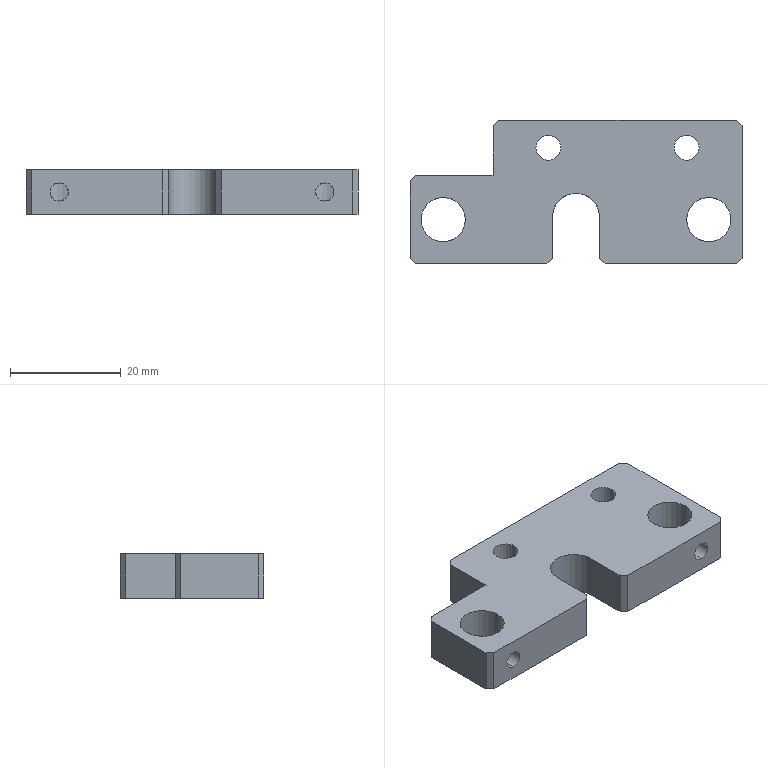Part | SolidWorks | features ICE 3, HoleWzd 2, Chamfer 1, Extrusion 1 | 1 solid | 31 faces | box 60 x 26 x 8 mm | volume 9318 mm3 | plane 18 | cylinder 13 | commonest cylinder face diameters 3.3 x4 4.5 x4 8 x4 8.5 x1
STEP:
#1=CARTESIAN_POINT('',(-2.75,21.,8.));
#2=VERTEX_POINT('',#1);
#3=CARTESIAN_POINT('',(-7.25,21.,8.));
#4=VERTEX_POINT('',#3);
#5=CARTESIAN_POINT('',(-5.,21.,8.));
#6=DIRECTION('',(0.,0.,-1.));
#7=DIRECTION('',(-1.,0.,0.));
#8=AXIS2_PLACEMENT_3D('',#5,#6,#7);
#9=CIRCLE('',#8,2.25);
#10=EDGE_CURVE('',#2,#4,#9,.T.);
#11=ORIENTED_EDGE('',*,*,#10,.F.);
#12=CARTESIAN_POINT('',(-2.75,21.,0.));
#13=VERTEX_POINT('',#12);
#14=CARTESIAN_POINT('',(-2.75,21.,8.));
#15=DIRECTION('',(0.,0.,-1.));
#16=VECTOR('',#15,1000.);
#17=LINE('',#14,#16);
#18=EDGE_CURVE('',#2,#13,#17,.T.);
#19=ORIENTED_EDGE('',*,*,#18,.T.);
#20=CARTESIAN_POINT('',(-7.25,21.,0.));
#21=VERTEX_POINT('',#20);
#22=CARTESIAN_POINT('',(-5.,21.,0.));
#23=DIRECTION('',(0.,0.,-1.));
#24=DIRECTION('',(-1.,0.,0.));
#25=AXIS2_PLACEMENT_3D('',#22,#23,#24);
#26=CIRCLE('',#25,2.25);
#27=EDGE_CURVE('',#13,#21,#26,.T.);
#28=ORIENTED_EDGE('',*,*,#27,.T.);
#29=CARTESIAN_POINT('',(-7.25,21.,8.));
#30=DIRECTION('',(0.,0.,-1.));
#31=VECTOR('',#30,1000.);
#32=LINE('',#29,#31);
#33=EDGE_CURVE('',#4,#21,#32,.T.);
#34=ORIENTED_EDGE('',*,*,#33,.F.);
#35=EDGE_LOOP('',(#11,#19,#28,#34));
#36=FACE_OUTER_BOUND('',#35,.T.);
#37=CARTESIAN_POINT('',(-5.,21.,8.));
#38=DIRECTION('',(0.,0.,-1.));
#39=DIRECTION('',(-1.,0.,0.));
#40=AXIS2_PLACEMENT_3D('',#37,#38,#39);
#41=CYLINDRICAL_SURFACE('',#40,2.25);
#42=ADVANCED_FACE('',(#36),#41,.F.);
#43=CARTESIAN_POINT('',(22.25,21.,8.));
#44=VERTEX_POINT('',#43);
#45=CARTESIAN_POINT('',(17.75,21.,8.));
#46=VERTEX_POINT('',#45);
#47=CARTESIAN_POINT('',(20.,21.,8.));
#48=DIRECTION('',(0.,0.,-1.));
#49=DIRECTION('',(-1.,0.,0.));
#50=AXIS2_PLACEMENT_3D('',#47,#48,#49);
#51=CIRCLE('',#50,2.25);
#52=EDGE_CURVE('',#44,#46,#51,.T.);
#53=ORIENTED_EDGE('',*,*,#52,.F.);
#54=CARTESIAN_POINT('',(22.25,21.,0.));
#55=VERTEX_POINT('',#54);
#56=CARTESIAN_POINT('',(22.25,21.,8.));
#57=DIRECTION('',(0.,0.,-1.));
#58=VECTOR('',#57,1000.);
#59=LINE('',#56,#58);
#60=EDGE_CURVE('',#44,#55,#59,.T.);
#61=ORIENTED_EDGE('',*,*,#60,.T.);
#62=CARTESIAN_POINT('',(17.75,21.,0.));
#63=VERTEX_POINT('',#62);
#64=CARTESIAN_POINT('',(20.,21.,0.));
#65=DIRECTION('',(0.,0.,-1.));
#66=DIRECTION('',(-1.,0.,0.));
#67=AXIS2_PLACEMENT_3D('',#64,#65,#66);
#68=CIRCLE('',#67,2.25);
#69=EDGE_CURVE('',#55,#63,#68,.T.);
#70=ORIENTED_EDGE('',*,*,#69,.T.);
#71=CARTESIAN_POINT('',(17.75,21.,8.));
#72=DIRECTION('',(0.,0.,-1.));
#73=VECTOR('',#72,1000.);
#74=LINE('',#71,#73);
#75=EDGE_CURVE('',#46,#63,#74,.T.);
#76=ORIENTED_EDGE('',*,*,#75,.F.);
#77=EDGE_LOOP('',(#53,#61,#70,#76));
#78=FACE_OUTER_BOUND('',#77,.T.);
#79=CARTESIAN_POINT('',(20.,21.,8.));
#80=DIRECTION('',(0.,0.,-1.));
#81=DIRECTION('',(-1.,0.,0.));
#82=AXIS2_PLACEMENT_3D('',#79,#80,#81);
#83=CYLINDRICAL_SURFACE('',#82,2.25);
#84=ADVANCED_FACE('',(#78),#83,.F.);
#85=CARTESIAN_POINT('',(-24.,4.,2.35));
#86=VERTEX_POINT('',#85);
#87=CARTESIAN_POINT('',(-24.,4.,5.65));
#88=VERTEX_POINT('',#87);
#89=CARTESIAN_POINT('',(-24.,4.,2.35));
#90=CARTESIAN_POINT('',(-24.11,4.,2.35));
#91=CARTESIAN_POINT('',(-24.219,4.005,2.361));
#92=CARTESIAN_POINT('',(-24.431,4.022,2.404));
#93=CARTESIAN_POINT('',(-24.537,4.035,2.436));
#94=CARTESIAN_POINT('',(-24.836,4.083,2.561));
#95=CARTESIAN_POINT('',(-25.017,4.128,2.684));
#96=CARTESIAN_POINT('',(-25.318,4.22,2.985));
#97=CARTESIAN_POINT('',(-25.44,4.267,3.166));
#98=CARTESIAN_POINT('',(-25.564,4.318,3.463));
#99=CARTESIAN_POINT('',(-25.596,4.332,3.568));
#100=CARTESIAN_POINT('',(-25.639,4.351,3.782));
#101=CARTESIAN_POINT('',(-25.65,4.356,3.89));
#102=CARTESIAN_POINT('',(-25.65,4.356,4.108));
#103=CARTESIAN_POINT('',(-25.639,4.351,4.219));
#104=CARTESIAN_POINT('',(-25.596,4.332,4.431));
#105=CARTESIAN_POINT('',(-25.565,4.318,4.535));
#106=CARTESIAN_POINT('',(-25.481,4.284,4.736));
#107=CARTESIAN_POINT('',(-25.43,4.264,4.83));
#108=CARTESIAN_POINT('',(-25.311,4.22,5.008));
#109=CARTESIAN_POINT('',(-25.242,4.197,5.092));
#110=CARTESIAN_POINT('',(-25.091,4.151,5.243));
#111=CARTESIAN_POINT('',(-25.009,4.128,5.31));
#112=CARTESIAN_POINT('',(-24.83,4.086,5.43));
#113=CARTESIAN_POINT('',(-24.734,4.067,5.481));
#114=CARTESIAN_POINT('',(-24.437,4.019,5.606));
#115=CARTESIAN_POINT('',(-24.217,4.,5.65));
#116=CARTESIAN_POINT('',(-24.,4.,5.65));
#117=B_SPLINE_CURVE_WITH_KNOTS('',3,(#89,#90,#91,#92,#93,#94,#95,#96,#97,#98,#99,#100,#101,#102,#103,#104,#105,#106,#107,#108,#109,#110,#111,#112,#113,#114,#115,#116),.UNSPECIFIED.,.F.,.F.,(4,2,2,2,2,2,2,2,2,2,2,2,2,4),(0.,0.0003261,0.0006522,0.001304,0.001957,0.002283,0.002609,0.002935,0.003261,0.003587,0.003913,0.004239,0.004565,0.005218),.UNSPECIFIED.);
#118=EDGE_CURVE('',#86,#88,#117,.T.);
#119=ORIENTED_EDGE('',*,*,#118,.T.);
#120=CARTESIAN_POINT('',(-24.,0.,5.65));
#121=VERTEX_POINT('',#120);
#122=CARTESIAN_POINT('',(-24.,0.,5.65));
#123=DIRECTION('',(0.,-1.,0.));
#124=VECTOR('',#123,1000.);
#125=LINE('',#122,#124);
#126=EDGE_CURVE('',#88,#121,#125,.T.);
#127=ORIENTED_EDGE('',*,*,#126,.T.);
#128=CARTESIAN_POINT('',(-24.,0.,2.35));
#129=VERTEX_POINT('',#128);
#130=CARTESIAN_POINT('',(-24.,0.,4.));
#131=DIRECTION('',(0.,-1.,0.));
#132=DIRECTION('',(0.,0.,-1.));
#133=AXIS2_PLACEMENT_3D('',#130,#131,#132);
#134=CIRCLE('',#133,1.65);
#135=EDGE_CURVE('',#121,#129,#134,.T.);
#136=ORIENTED_EDGE('',*,*,#135,.T.);
#137=CARTESIAN_POINT('',(-24.,0.,2.35));
#138=DIRECTION('',(0.,-1.,0.));
#139=VECTOR('',#138,1000.);
#140=LINE('',#137,#139);
#141=EDGE_CURVE('',#86,#129,#140,.T.);
#142=ORIENTED_EDGE('',*,*,#141,.F.);
#143=EDGE_LOOP('',(#119,#127,#136,#142));
#144=FACE_OUTER_BOUND('',#143,.T.);
#145=CARTESIAN_POINT('',(-24.,0.,4.));
#146=DIRECTION('',(0.,-1.,0.));
#147=DIRECTION('',(0.,0.,-1.));
#148=AXIS2_PLACEMENT_3D('',#145,#146,#147);
#149=CYLINDRICAL_SURFACE('',#148,1.65);
#150=ADVANCED_FACE('',(#144),#149,.F.);
#151=CARTESIAN_POINT('',(24.,4.,2.35));
#152=VERTEX_POINT('',#151);
#153=CARTESIAN_POINT('',(24.,4.,5.65));
#154=VERTEX_POINT('',#153);
#155=CARTESIAN_POINT('',(24.,4.,2.35));
#156=CARTESIAN_POINT('',(23.89,4.,2.35));
#157=CARTESIAN_POINT('',(23.781,4.005,2.361));
#158=CARTESIAN_POINT('',(23.569,4.022,2.404));
#159=CARTESIAN_POINT('',(23.463,4.035,2.436));
#160=CARTESIAN_POINT('',(23.164,4.083,2.561));
#161=CARTESIAN_POINT('',(22.983,4.128,2.684));
#162=CARTESIAN_POINT('',(22.682,4.22,2.985));
#163=CARTESIAN_POINT('',(22.56,4.267,3.166));
#164=CARTESIAN_POINT('',(22.436,4.318,3.463));
#165=CARTESIAN_POINT('',(22.404,4.332,3.568));
#166=CARTESIAN_POINT('',(22.361,4.351,3.782));
#167=CARTESIAN_POINT('',(22.35,4.356,3.89));
#168=CARTESIAN_POINT('',(22.35,4.356,4.108));
#169=CARTESIAN_POINT('',(22.361,4.351,4.219));
#170=CARTESIAN_POINT('',(22.404,4.332,4.431));
#171=CARTESIAN_POINT('',(22.435,4.318,4.535));
#172=CARTESIAN_POINT('',(22.519,4.284,4.736));
#173=CARTESIAN_POINT('',(22.57,4.264,4.83));
#174=CARTESIAN_POINT('',(22.689,4.22,5.008));
#175=CARTESIAN_POINT('',(22.758,4.197,5.092));
#176=CARTESIAN_POINT('',(22.909,4.151,5.243));
#177=CARTESIAN_POINT('',(22.991,4.128,5.31));
#178=CARTESIAN_POINT('',(23.17,4.086,5.43));
#179=CARTESIAN_POINT('',(23.266,4.067,5.481));
#180=CARTESIAN_POINT('',(23.563,4.019,5.606));
#181=CARTESIAN_POINT('',(23.783,4.,5.65));
#182=CARTESIAN_POINT('',(24.,4.,5.65));
#183=B_SPLINE_CURVE_WITH_KNOTS('',3,(#155,#156,#157,#158,#159,#160,#161,#162,#163,#164,#165,#166,#167,#168,#169,#170,#171,#172,#173,#174,#175,#176,#177,#178,#179,#180,#181,#182),.UNSPECIFIED.,.F.,.F.,(4,2,2,2,2,2,2,2,2,2,2,2,2,4),(0.,0.0003261,0.0006522,0.001304,0.001957,0.002283,0.002609,0.002935,0.003261,0.003587,0.003913,0.004239,0.004565,0.005218),.UNSPECIFIED.);
#184=EDGE_CURVE('',#152,#154,#183,.T.);
#185=ORIENTED_EDGE('',*,*,#184,.T.);
#186=CARTESIAN_POINT('',(24.,0.,5.65));
#187=VERTEX_POINT('',#186);
#188=CARTESIAN_POINT('',(24.,0.,5.65));
#189=DIRECTION('',(0.,-1.,0.));
#190=VECTOR('',#189,1000.);
#191=LINE('',#188,#190);
#192=EDGE_CURVE('',#154,#187,#191,.T.);
#193=ORIENTED_EDGE('',*,*,#192,.T.);
#194=CARTESIAN_POINT('',(24.,0.,2.35));
#195=VERTEX_POINT('',#194);
#196=CARTESIAN_POINT('',(24.,0.,4.));
#197=DIRECTION('',(0.,-1.,0.));
#198=DIRECTION('',(0.,0.,-1.));
#199=AXIS2_PLACEMENT_3D('',#196,#197,#198);
#200=CIRCLE('',#199,1.65);
#201=EDGE_CURVE('',#187,#195,#200,.T.);
#202=ORIENTED_EDGE('',*,*,#201,.T.);
#203=CARTESIAN_POINT('',(24.,0.,2.35));
#204=DIRECTION('',(0.,-1.,0.));
#205=VECTOR('',#204,1000.);
#206=LINE('',#203,#205);
#207=EDGE_CURVE('',#152,#195,#206,.T.);
#208=ORIENTED_EDGE('',*,*,#207,.F.);
#209=EDGE_LOOP('',(#185,#193,#202,#208));
#210=FACE_OUTER_BOUND('',#209,.T.);
#211=CARTESIAN_POINT('',(24.,0.,4.));
#212=DIRECTION('',(0.,-1.,0.));
#213=DIRECTION('',(0.,0.,-1.));
#214=AXIS2_PLACEMENT_3D('',#211,#212,#213);
#215=CYLINDRICAL_SURFACE('',#214,1.65);
#216=ADVANCED_FACE('',(#210),#215,.F.);
#217=ORIENTED_EDGE('',*,*,#184,.F.);
#218=CARTESIAN_POINT('',(24.,4.,5.65));
#219=CARTESIAN_POINT('',(24.109,4.,5.65));
#220=CARTESIAN_POINT('',(24.219,4.005,5.639));
#221=CARTESIAN_POINT('',(24.433,4.022,5.596));
#222=CARTESIAN_POINT('',(24.536,4.035,5.564));
#223=CARTESIAN_POINT('',(24.835,4.083,5.439));
#224=CARTESIAN_POINT('',(25.016,4.128,5.318));
#225=CARTESIAN_POINT('',(25.244,4.197,5.09));
#226=CARTESIAN_POINT('',(25.311,4.22,5.008));
#227=CARTESIAN_POINT('',(25.43,4.264,4.83));
#228=CARTESIAN_POINT('',(25.481,4.284,4.734));
#229=CARTESIAN_POINT('',(25.564,4.318,4.535));
#230=CARTESIAN_POINT('',(25.596,4.332,4.433));
#231=CARTESIAN_POINT('',(25.639,4.351,4.22));
#232=CARTESIAN_POINT('',(25.65,4.356,4.109));
#233=CARTESIAN_POINT('',(25.65,4.356,3.783));
#234=CARTESIAN_POINT('',(25.606,4.335,3.564));
#235=CARTESIAN_POINT('',(25.482,4.284,3.266));
#236=CARTESIAN_POINT('',(25.43,4.264,3.17));
#237=CARTESIAN_POINT('',(25.311,4.22,2.992));
#238=CARTESIAN_POINT('',(25.243,4.197,2.91));
#239=CARTESIAN_POINT('',(25.092,4.151,2.758));
#240=CARTESIAN_POINT('',(25.008,4.128,2.689));
#241=CARTESIAN_POINT('',(24.831,4.086,2.571));
#242=CARTESIAN_POINT('',(24.737,4.067,2.52));
#243=CARTESIAN_POINT('',(24.435,4.018,2.393));
#244=CARTESIAN_POINT('',(24.221,4.,2.35));
#245=CARTESIAN_POINT('',(24.,4.,2.35));
#246=B_SPLINE_CURVE_WITH_KNOTS('',3,(#218,#219,#220,#221,#222,#223,#224,#225,#226,#227,#228,#229,#230,#231,#232,#233,#234,#235,#236,#237,#238,#239,#240,#241,#242,#243,#244,#245),.UNSPECIFIED.,.F.,.F.,(4,2,2,2,2,2,2,2,2,2,2,2,2,4),(0.005218,0.005543,0.005869,0.006521,0.006847,0.007173,0.007499,0.007824,0.008476,0.008802,0.009128,0.009454,0.009779,0.01043),.UNSPECIFIED.);
#247=EDGE_CURVE('',#154,#152,#246,.T.);
#248=ORIENTED_EDGE('',*,*,#247,.F.);
#249=EDGE_LOOP('',(#217,#248));
#250=FACE_BOUND('',#249,.T.);
#251=CARTESIAN_POINT('',(20.,8.,8.));
#252=VERTEX_POINT('',#251);
#253=CARTESIAN_POINT('',(28.,8.,8.));
#254=VERTEX_POINT('',#253);
#255=CARTESIAN_POINT('',(24.,8.,8.));
#256=DIRECTION('',(0.,0.,1.));
#257=DIRECTION('',(-1.,0.,0.));
#258=AXIS2_PLACEMENT_3D('',#255,#256,#257);
#259=CIRCLE('',#258,4.);
#260=EDGE_CURVE('',#252,#254,#259,.T.);
#261=ORIENTED_EDGE('',*,*,#260,.T.);
#262=CARTESIAN_POINT('',(28.,8.,0.));
#263=VERTEX_POINT('',#262);
#264=CARTESIAN_POINT('',(28.,8.,8.));
#265=DIRECTION('',(0.,0.,-1.));
#266=VECTOR('',#265,1000.);
#267=LINE('',#264,#266);
#268=EDGE_CURVE('',#254,#263,#267,.T.);
#269=ORIENTED_EDGE('',*,*,#268,.T.);
#270=CARTESIAN_POINT('',(20.,8.,0.));
#271=VERTEX_POINT('',#270);
#272=CARTESIAN_POINT('',(24.,8.,0.));
#273=DIRECTION('',(0.,0.,1.));
#274=DIRECTION('',(-1.,0.,0.));
#275=AXIS2_PLACEMENT_3D('',#272,#273,#274);
#276=CIRCLE('',#275,4.);
#277=EDGE_CURVE('',#271,#263,#276,.T.);
#278=ORIENTED_EDGE('',*,*,#277,.F.);
#279=CARTESIAN_POINT('',(20.,8.,8.));
#280=DIRECTION('',(0.,0.,-1.));
#281=VECTOR('',#280,1000.);
#282=LINE('',#279,#281);
#283=EDGE_CURVE('',#252,#271,#282,.T.);
#284=ORIENTED_EDGE('',*,*,#283,.F.);
#285=EDGE_LOOP('',(#261,#269,#278,#284));
#286=FACE_OUTER_BOUND('',#285,.T.);
#287=CARTESIAN_POINT('',(24.,8.,8.));
#288=DIRECTION('',(0.,0.,-1.));
#289=DIRECTION('',(-1.,0.,0.));
#290=AXIS2_PLACEMENT_3D('',#287,#288,#289);
#291=CYLINDRICAL_SURFACE('',#290,4.);
#292=ADVANCED_FACE('',(#250,#286),#291,.F.);
#293=ORIENTED_EDGE('',*,*,#118,.F.);
#294=CARTESIAN_POINT('',(-24.,4.,5.65));
#295=CARTESIAN_POINT('',(-23.891,4.,5.65));
#296=CARTESIAN_POINT('',(-23.781,4.005,5.639));
#297=CARTESIAN_POINT('',(-23.567,4.022,5.596));
#298=CARTESIAN_POINT('',(-23.464,4.035,5.564));
#299=CARTESIAN_POINT('',(-23.165,4.083,5.439));
#300=CARTESIAN_POINT('',(-22.984,4.128,5.318));
#301=CARTESIAN_POINT('',(-22.756,4.197,5.09));
#302=CARTESIAN_POINT('',(-22.689,4.22,5.008));
#303=CARTESIAN_POINT('',(-22.57,4.264,4.83));
#304=CARTESIAN_POINT('',(-22.519,4.284,4.734));
#305=CARTESIAN_POINT('',(-22.436,4.318,4.535));
#306=CARTESIAN_POINT('',(-22.404,4.332,4.433));
#307=CARTESIAN_POINT('',(-22.361,4.351,4.22));
#308=CARTESIAN_POINT('',(-22.35,4.356,4.109));
#309=CARTESIAN_POINT('',(-22.35,4.356,3.783));
#310=CARTESIAN_POINT('',(-22.394,4.335,3.564));
#311=CARTESIAN_POINT('',(-22.518,4.284,3.266));
#312=CARTESIAN_POINT('',(-22.57,4.264,3.17));
#313=CARTESIAN_POINT('',(-22.689,4.22,2.992));
#314=CARTESIAN_POINT('',(-22.757,4.197,2.91));
#315=CARTESIAN_POINT('',(-22.908,4.151,2.758));
#316=CARTESIAN_POINT('',(-22.992,4.128,2.689));
#317=CARTESIAN_POINT('',(-23.169,4.086,2.571));
#318=CARTESIAN_POINT('',(-23.263,4.067,2.52));
#319=CARTESIAN_POINT('',(-23.565,4.018,2.393));
#320=CARTESIAN_POINT('',(-23.779,4.,2.35));
#321=CARTESIAN_POINT('',(-24.,4.,2.35));
#322=B_SPLINE_CURVE_WITH_KNOTS('',3,(#294,#295,#296,#297,#298,#299,#300,#301,#302,#303,#304,#305,#306,#307,#308,#309,#310,#311,#312,#313,#314,#315,#316,#317,#318,#319,#320,#321),.UNSPECIFIED.,.F.,.F.,(4,2,2,2,2,2,2,2,2,2,2,2,2,4),(0.005218,0.005543,0.005869,0.006521,0.006847,0.007173,0.007499,0.007824,0.008476,0.008802,0.009128,0.009454,0.009779,0.01043),.UNSPECIFIED.);
#323=EDGE_CURVE('',#88,#86,#322,.T.);
#324=ORIENTED_EDGE('',*,*,#323,.F.);
#325=EDGE_LOOP('',(#293,#324));
#326=FACE_BOUND('',#325,.T.);
#327=CARTESIAN_POINT('',(-28.,8.,8.));
#328=VERTEX_POINT('',#327);
#329=CARTESIAN_POINT('',(-20.,8.,8.));
#330=VERTEX_POINT('',#329);
#331=CARTESIAN_POINT('',(-24.,8.,8.));
#332=DIRECTION('',(0.,0.,1.));
#333=DIRECTION('',(1.,0.,0.));
#334=AXIS2_PLACEMENT_3D('',#331,#332,#333);
#335=CIRCLE('',#334,4.);
#336=EDGE_CURVE('',#328,#330,#335,.T.);
#337=ORIENTED_EDGE('',*,*,#336,.T.);
#338=CARTESIAN_POINT('',(-20.,8.,0.));
#339=VERTEX_POINT('',#338);
#340=CARTESIAN_POINT('',(-20.,8.,8.));
#341=DIRECTION('',(0.,0.,-1.));
#342=VECTOR('',#341,1000.);
#343=LINE('',#340,#342);
#344=EDGE_CURVE('',#330,#339,#343,.T.);
#345=ORIENTED_EDGE('',*,*,#344,.T.);
#346=CARTESIAN_POINT('',(-28.,8.,0.));
#347=VERTEX_POINT('',#346);
#348=CARTESIAN_POINT('',(-24.,8.,0.));
#349=DIRECTION('',(0.,0.,1.));
#350=DIRECTION('',(1.,0.,0.));
#351=AXIS2_PLACEMENT_3D('',#348,#349,#350);
#352=CIRCLE('',#351,4.);
#353=EDGE_CURVE('',#347,#339,#352,.T.);
#354=ORIENTED_EDGE('',*,*,#353,.F.);
#355=CARTESIAN_POINT('',(-28.,8.,8.));
#356=DIRECTION('',(0.,0.,-1.));
#357=VECTOR('',#356,1000.);
#358=LINE('',#355,#357);
#359=EDGE_CURVE('',#328,#347,#358,.T.);
#360=ORIENTED_EDGE('',*,*,#359,.F.);
#361=EDGE_LOOP('',(#337,#345,#354,#360));
#362=FACE_OUTER_BOUND('',#361,.T.);
#363=CARTESIAN_POINT('',(-24.,8.,8.));
#364=DIRECTION('',(0.,0.,-1.));
#365=DIRECTION('',(-1.,0.,0.));
#366=AXIS2_PLACEMENT_3D('',#363,#364,#365);
#367=CYLINDRICAL_SURFACE('',#366,4.);
#368=ADVANCED_FACE('',(#326,#362),#367,.F.);
#369=CARTESIAN_POINT('',(-24.,0.,4.));
#370=DIRECTION('',(0.,-1.,0.));
#371=DIRECTION('',(0.,0.,-1.));
#372=AXIS2_PLACEMENT_3D('',#369,#370,#371);
#373=CIRCLE('',#372,1.65);
#374=EDGE_CURVE('',#129,#121,#373,.T.);
#375=ORIENTED_EDGE('',*,*,#374,.F.);
#376=ORIENTED_EDGE('',*,*,#135,.F.);
#377=EDGE_LOOP('',(#375,#376));
#378=FACE_BOUND('',#377,.T.);
#379=CARTESIAN_POINT('',(-29.,0.,8.));
#380=VERTEX_POINT('',#379);
#381=CARTESIAN_POINT('',(-5.25,0.,8.));
#382=VERTEX_POINT('',#381);
#383=CARTESIAN_POINT('',(30.,0.,8.));
#384=DIRECTION('',(1.,0.,0.));
#385=VECTOR('',#384,1000.);
#386=LINE('',#383,#385);
#387=EDGE_CURVE('',#380,#382,#386,.T.);
#388=ORIENTED_EDGE('',*,*,#387,.F.);
#389=CARTESIAN_POINT('',(-29.,0.,0.));
#390=VERTEX_POINT('',#389);
#391=CARTESIAN_POINT('',(-29.,0.,8.));
#392=DIRECTION('',(0.,0.,-1.));
#393=VECTOR('',#392,1000.);
#394=LINE('',#391,#393);
#395=EDGE_CURVE('',#380,#390,#394,.T.);
#396=ORIENTED_EDGE('',*,*,#395,.T.);
#397=CARTESIAN_POINT('',(-5.25,0.,0.));
#398=VERTEX_POINT('',#397);
#399=CARTESIAN_POINT('',(30.,0.,0.));
#400=DIRECTION('',(1.,0.,0.));
#401=VECTOR('',#400,1000.);
#402=LINE('',#399,#401);
#403=EDGE_CURVE('',#390,#398,#402,.T.);
#404=ORIENTED_EDGE('',*,*,#403,.T.);
#405=CARTESIAN_POINT('',(-5.25,0.,8.));
#406=DIRECTION('',(0.,0.,1.));
#407=VECTOR('',#406,1000.);
#408=LINE('',#405,#407);
#409=EDGE_CURVE('',#398,#382,#408,.T.);
#410=ORIENTED_EDGE('',*,*,#409,.T.);
#411=EDGE_LOOP('',(#388,#396,#404,#410));
#412=FACE_OUTER_BOUND('',#411,.T.);
#413=CARTESIAN_POINT('',(30.,0.,8.));
#414=DIRECTION('',(0.,1.,0.));
#415=DIRECTION('',(0.,0.,1.));
#416=AXIS2_PLACEMENT_3D('',#413,#414,#415);
#417=PLANE('',#416);
#418=ADVANCED_FACE('',(#378,#412),#417,.F.);
#419=CARTESIAN_POINT('',(-5.,21.,8.));
#420=DIRECTION('',(0.,0.,-1.));
#421=DIRECTION('',(-1.,0.,0.));
#422=AXIS2_PLACEMENT_3D('',#419,#420,#421);
#423=CIRCLE('',#422,2.25);
#424=EDGE_CURVE('',#4,#2,#423,.T.);
#425=ORIENTED_EDGE('',*,*,#424,.T.);
#426=ORIENTED_EDGE('',*,*,#10,.T.);
#427=EDGE_LOOP('',(#425,#426));
#428=FACE_BOUND('',#427,.T.);
#429=CARTESIAN_POINT('',(20.,21.,8.));
#430=DIRECTION('',(0.,0.,-1.));
#431=DIRECTION('',(-1.,0.,0.));
#432=AXIS2_PLACEMENT_3D('',#429,#430,#431);
#433=CIRCLE('',#432,2.25);
#434=EDGE_CURVE('',#46,#44,#433,.T.);
#435=ORIENTED_EDGE('',*,*,#434,.T.);
#436=ORIENTED_EDGE('',*,*,#52,.T.);
#437=EDGE_LOOP('',(#435,#436));
#438=FACE_BOUND('',#437,.T.);
#439=CARTESIAN_POINT('',(30.,1.,8.));
#440=VERTEX_POINT('',#439);
#441=CARTESIAN_POINT('',(30.,25.,8.));
#442=VERTEX_POINT('',#441);
#443=CARTESIAN_POINT('',(30.,0.,8.));
#444=DIRECTION('',(0.,1.,0.));
#445=VECTOR('',#444,1000.);
#446=LINE('',#443,#445);
#447=EDGE_CURVE('',#440,#442,#446,.T.);
#448=ORIENTED_EDGE('',*,*,#447,.T.);
#449=CARTESIAN_POINT('',(29.,26.,8.));
#450=VERTEX_POINT('',#449);
#451=CARTESIAN_POINT('',(29.5,25.5,8.));
#452=DIRECTION('',(-0.7071,0.7071,0.));
#453=VECTOR('',#452,1000.);
#454=LINE('',#451,#453);
#455=EDGE_CURVE('',#442,#450,#454,.T.);
#456=ORIENTED_EDGE('',*,*,#455,.T.);
#457=CARTESIAN_POINT('',(-14.,26.,8.));
#458=VERTEX_POINT('',#457);
#459=CARTESIAN_POINT('',(30.,26.,8.));
#460=DIRECTION('',(-1.,0.,0.));
#461=VECTOR('',#460,1000.);
#462=LINE('',#459,#461);
#463=EDGE_CURVE('',#450,#458,#462,.T.);
#464=ORIENTED_EDGE('',*,*,#463,.T.);
#465=CARTESIAN_POINT('',(-15.,25.,8.));
#466=VERTEX_POINT('',#465);
#467=CARTESIAN_POINT('',(8.,48.,8.));
#468=DIRECTION('',(-0.7071,-0.7071,0.));
#469=VECTOR('',#468,1000.);
#470=LINE('',#467,#469);
#471=EDGE_CURVE('',#458,#466,#470,.T.);
#472=ORIENTED_EDGE('',*,*,#471,.T.);
#473=CARTESIAN_POINT('',(-15.,16.,8.));
#474=VERTEX_POINT('',#473);
#475=CARTESIAN_POINT('',(-15.,26.,8.));
#476=DIRECTION('',(0.,-1.,0.));
#477=VECTOR('',#476,1000.);
#478=LINE('',#475,#477);
#479=EDGE_CURVE('',#466,#474,#478,.T.);
#480=ORIENTED_EDGE('',*,*,#479,.T.);
#481=CARTESIAN_POINT('',(-29.,16.,8.));
#482=VERTEX_POINT('',#481);
#483=CARTESIAN_POINT('',(-15.,16.,8.));
#484=DIRECTION('',(-1.,0.,0.));
#485=VECTOR('',#484,1000.);
#486=LINE('',#483,#485);
#487=EDGE_CURVE('',#474,#482,#486,.T.);
#488=ORIENTED_EDGE('',*,*,#487,.T.);
#489=CARTESIAN_POINT('',(-30.,15.,8.));
#490=VERTEX_POINT('',#489);
#491=CARTESIAN_POINT('',(5.5,50.5,8.));
#492=DIRECTION('',(-0.7071,-0.7071,0.));
#493=VECTOR('',#492,1000.);
#494=LINE('',#491,#493);
#495=EDGE_CURVE('',#482,#490,#494,.T.);
#496=ORIENTED_EDGE('',*,*,#495,.T.);
#497=CARTESIAN_POINT('',(-30.,1.,8.));
#498=VERTEX_POINT('',#497);
#499=CARTESIAN_POINT('',(-30.,0.,8.));
#500=DIRECTION('',(0.,-1.,0.));
#501=VECTOR('',#500,1000.);
#502=LINE('',#499,#501);
#503=EDGE_CURVE('',#490,#498,#502,.T.);
#504=ORIENTED_EDGE('',*,*,#503,.T.);
#505=CARTESIAN_POINT('',(-12.5,-16.5,8.));
#506=DIRECTION('',(0.7071,-0.7071,0.));
#507=VECTOR('',#506,1000.);
#508=LINE('',#505,#507);
#509=EDGE_CURVE('',#498,#380,#508,.T.);
#510=ORIENTED_EDGE('',*,*,#509,.T.);
#511=ORIENTED_EDGE('',*,*,#387,.T.);
#512=CARTESIAN_POINT('',(-4.25,1.,8.));
#513=VERTEX_POINT('',#512);
#514=CARTESIAN_POINT('',(25.375,30.625,8.));
#515=DIRECTION('',(0.7071,0.7071,0.));
#516=VECTOR('',#515,1000.);
#517=LINE('',#514,#516);
#518=EDGE_CURVE('',#382,#513,#517,.T.);
#519=ORIENTED_EDGE('',*,*,#518,.T.);
#520=CARTESIAN_POINT('',(-4.25,8.5,8.));
#521=VERTEX_POINT('',#520);
#522=CARTESIAN_POINT('',(-4.25,0.,8.));
#523=DIRECTION('',(0.,-1.,0.));
#524=VECTOR('',#523,1000.);
#525=LINE('',#522,#524);
#526=EDGE_CURVE('',#521,#513,#525,.T.);
#527=ORIENTED_EDGE('',*,*,#526,.F.);
#528=CARTESIAN_POINT('',(4.25,8.5,8.));
#529=VERTEX_POINT('',#528);
#530=CARTESIAN_POINT('',(0.,8.5,8.));
#531=DIRECTION('',(0.,0.,1.));
#532=DIRECTION('',(1.,0.,0.));
#533=AXIS2_PLACEMENT_3D('',#530,#531,#532);
#534=CIRCLE('',#533,4.25);
#535=EDGE_CURVE('',#529,#521,#534,.T.);
#536=ORIENTED_EDGE('',*,*,#535,.F.);
#537=CARTESIAN_POINT('',(4.25,1.,8.));
#538=VERTEX_POINT('',#537);
#539=CARTESIAN_POINT('',(4.25,0.,8.));
#540=DIRECTION('',(0.,1.,0.));
#541=VECTOR('',#540,1000.);
#542=LINE('',#539,#541);
#543=EDGE_CURVE('',#538,#529,#542,.T.);
#544=ORIENTED_EDGE('',*,*,#543,.F.);
#545=CARTESIAN_POINT('',(5.25,0.,8.));
#546=VERTEX_POINT('',#545);
#547=CARTESIAN_POINT('',(4.625,0.625,8.));
#548=DIRECTION('',(0.7071,-0.7071,0.));
#549=VECTOR('',#548,1000.);
#550=LINE('',#547,#549);
#551=EDGE_CURVE('',#538,#546,#550,.T.);
#552=ORIENTED_EDGE('',*,*,#551,.T.);
#553=CARTESIAN_POINT('',(29.,0.,8.));
#554=VERTEX_POINT('',#553);
#555=CARTESIAN_POINT('',(30.,0.,8.));
#556=DIRECTION('',(1.,0.,0.));
#557=VECTOR('',#556,1000.);
#558=LINE('',#555,#557);
#559=EDGE_CURVE('',#546,#554,#558,.T.);
#560=ORIENTED_EDGE('',*,*,#559,.T.);
#561=CARTESIAN_POINT('',(42.5,13.5,8.));
#562=DIRECTION('',(0.7071,0.7071,0.));
#563=VECTOR('',#562,1000.);
#564=LINE('',#561,#563);
#565=EDGE_CURVE('',#554,#440,#564,.T.);
#566=ORIENTED_EDGE('',*,*,#565,.T.);
#567=EDGE_LOOP('',(#448,#456,#464,#472,#480,#488,#496,#504,#510,#511,#519,#527,#536,#544,#552,#560,#566));
#568=FACE_OUTER_BOUND('',#567,.T.);
#569=ORIENTED_EDGE('',*,*,#336,.F.);
#570=CARTESIAN_POINT('',(-24.,8.,8.));
#571=DIRECTION('',(0.,0.,1.));
#572=DIRECTION('',(1.,0.,0.));
#573=AXIS2_PLACEMENT_3D('',#570,#571,#572);
#574=CIRCLE('',#573,4.);
#575=EDGE_CURVE('',#330,#328,#574,.T.);
#576=ORIENTED_EDGE('',*,*,#575,.F.);
#577=EDGE_LOOP('',(#569,#576));
#578=FACE_BOUND('',#577,.T.);
#579=ORIENTED_EDGE('',*,*,#260,.F.);
#580=CARTESIAN_POINT('',(24.,8.,8.));
#581=DIRECTION('',(0.,0.,1.));
#582=DIRECTION('',(-1.,0.,0.));
#583=AXIS2_PLACEMENT_3D('',#580,#581,#582);
#584=CIRCLE('',#583,4.);
#585=EDGE_CURVE('',#254,#252,#584,.T.);
#586=ORIENTED_EDGE('',*,*,#585,.F.);
#587=EDGE_LOOP('',(#579,#586));
#588=FACE_BOUND('',#587,.T.);
#589=CARTESIAN_POINT('',(30.,26.,8.));
#590=DIRECTION('',(0.,0.,1.));
#591=DIRECTION('',(1.,0.,0.));
#592=AXIS2_PLACEMENT_3D('',#589,#590,#591);
#593=PLANE('',#592);
#594=ADVANCED_FACE('',(#428,#438,#568,#578,#588),#593,.T.);
#595=CARTESIAN_POINT('',(-5.,21.,0.));
#596=DIRECTION('',(0.,0.,-1.));
#597=DIRECTION('',(-1.,0.,0.));
#598=AXIS2_PLACEMENT_3D('',#595,#596,#597);
#599=CIRCLE('',#598,2.25);
#600=EDGE_CURVE('',#21,#13,#599,.T.);
#601=ORIENTED_EDGE('',*,*,#600,.F.);
#602=ORIENTED_EDGE('',*,*,#27,.F.);
#603=EDGE_LOOP('',(#601,#602));
#604=FACE_BOUND('',#603,.T.);
#605=CARTESIAN_POINT('',(20.,21.,0.));
#606=DIRECTION('',(0.,0.,-1.));
#607=DIRECTION('',(-1.,0.,0.));
#608=AXIS2_PLACEMENT_3D('',#605,#606,#607);
#609=CIRCLE('',#608,2.25);
#610=EDGE_CURVE('',#63,#55,#609,.T.);
#611=ORIENTED_EDGE('',*,*,#610,.F.);
#612=ORIENTED_EDGE('',*,*,#69,.F.);
#613=EDGE_LOOP('',(#611,#612));
#614=FACE_BOUND('',#613,.T.);
#615=ORIENTED_EDGE('',*,*,#353,.T.);
#616=CARTESIAN_POINT('',(-24.,8.,0.));
#617=DIRECTION('',(0.,0.,1.));
#618=DIRECTION('',(1.,0.,0.));
#619=AXIS2_PLACEMENT_3D('',#616,#617,#618);
#620=CIRCLE('',#619,4.);
#621=EDGE_CURVE('',#339,#347,#620,.T.);
#622=ORIENTED_EDGE('',*,*,#621,.T.);
#623=EDGE_LOOP('',(#615,#622));
#624=FACE_BOUND('',#623,.T.);
#625=CARTESIAN_POINT('',(29.,26.,0.));
#626=VERTEX_POINT('',#625);
#627=CARTESIAN_POINT('',(-14.,26.,0.));
#628=VERTEX_POINT('',#627);
#629=CARTESIAN_POINT('',(30.,26.,0.));
#630=DIRECTION('',(-1.,0.,0.));
#631=VECTOR('',#630,1000.);
#632=LINE('',#629,#631);
#633=EDGE_CURVE('',#626,#628,#632,.T.);
#634=ORIENTED_EDGE('',*,*,#633,.F.);
#635=CARTESIAN_POINT('',(30.,25.,0.));
#636=VERTEX_POINT('',#635);
#637=CARTESIAN_POINT('',(29.,26.,0.));
#638=DIRECTION('',(0.7071,-0.7071,0.));
#639=VECTOR('',#638,1000.);
#640=LINE('',#637,#639);
#641=EDGE_CURVE('',#626,#636,#640,.T.);
#642=ORIENTED_EDGE('',*,*,#641,.T.);
#643=CARTESIAN_POINT('',(30.,1.,0.));
#644=VERTEX_POINT('',#643);
#645=CARTESIAN_POINT('',(30.,0.,0.));
#646=DIRECTION('',(0.,1.,0.));
#647=VECTOR('',#646,1000.);
#648=LINE('',#645,#647);
#649=EDGE_CURVE('',#644,#636,#648,.T.);
#650=ORIENTED_EDGE('',*,*,#649,.F.);
#651=CARTESIAN_POINT('',(29.,0.,0.));
#652=VERTEX_POINT('',#651);
#653=CARTESIAN_POINT('',(30.,1.,0.));
#654=DIRECTION('',(-0.7071,-0.7071,0.));
#655=VECTOR('',#654,1000.);
#656=LINE('',#653,#655);
#657=EDGE_CURVE('',#644,#652,#656,.T.);
#658=ORIENTED_EDGE('',*,*,#657,.T.);
#659=CARTESIAN_POINT('',(5.25,0.,0.));
#660=VERTEX_POINT('',#659);
#661=CARTESIAN_POINT('',(30.,0.,0.));
#662=DIRECTION('',(1.,0.,0.));
#663=VECTOR('',#662,1000.);
#664=LINE('',#661,#663);
#665=EDGE_CURVE('',#660,#652,#664,.T.);
#666=ORIENTED_EDGE('',*,*,#665,.F.);
#667=CARTESIAN_POINT('',(4.25,1.,0.));
#668=VERTEX_POINT('',#667);
#669=CARTESIAN_POINT('',(4.25,1.,0.));
#670=DIRECTION('',(-0.7071,0.7071,0.));
#671=VECTOR('',#670,1000.);
#672=LINE('',#669,#671);
#673=EDGE_CURVE('',#660,#668,#672,.T.);
#674=ORIENTED_EDGE('',*,*,#673,.T.);
#675=CARTESIAN_POINT('',(4.25,8.5,0.));
#676=VERTEX_POINT('',#675);
#677=CARTESIAN_POINT('',(4.25,0.,0.));
#678=DIRECTION('',(0.,1.,0.));
#679=VECTOR('',#678,1000.);
#680=LINE('',#677,#679);
#681=EDGE_CURVE('',#668,#676,#680,.T.);
#682=ORIENTED_EDGE('',*,*,#681,.T.);
#683=CARTESIAN_POINT('',(-4.25,8.5,0.));
#684=VERTEX_POINT('',#683);
#685=CARTESIAN_POINT('',(0.,8.5,0.));
#686=DIRECTION('',(0.,0.,1.));
#687=DIRECTION('',(1.,0.,0.));
#688=AXIS2_PLACEMENT_3D('',#685,#686,#687);
#689=CIRCLE('',#688,4.25);
#690=EDGE_CURVE('',#676,#684,#689,.T.);
#691=ORIENTED_EDGE('',*,*,#690,.T.);
#692=CARTESIAN_POINT('',(-4.25,1.,0.));
#693=VERTEX_POINT('',#692);
#694=CARTESIAN_POINT('',(-4.25,0.,0.));
#695=DIRECTION('',(0.,-1.,0.));
#696=VECTOR('',#695,1000.);
#697=LINE('',#694,#696);
#698=EDGE_CURVE('',#684,#693,#697,.T.);
#699=ORIENTED_EDGE('',*,*,#698,.T.);
#700=CARTESIAN_POINT('',(-5.25,0.,0.));
#701=DIRECTION('',(-0.7071,-0.7071,0.));
#702=VECTOR('',#701,1000.);
#703=LINE('',#700,#702);
#704=EDGE_CURVE('',#693,#398,#703,.T.);
#705=ORIENTED_EDGE('',*,*,#704,.T.);
#706=ORIENTED_EDGE('',*,*,#403,.F.);
#707=CARTESIAN_POINT('',(-30.,1.,0.));
#708=VERTEX_POINT('',#707);
#709=CARTESIAN_POINT('',(-29.,0.,0.));
#710=DIRECTION('',(-0.7071,0.7071,0.));
#711=VECTOR('',#710,1000.);
#712=LINE('',#709,#711);
#713=EDGE_CURVE('',#390,#708,#712,.T.);
#714=ORIENTED_EDGE('',*,*,#713,.T.);
#715=CARTESIAN_POINT('',(-30.,15.,0.));
#716=VERTEX_POINT('',#715);
#717=CARTESIAN_POINT('',(-30.,0.,0.));
#718=DIRECTION('',(0.,-1.,0.));
#719=VECTOR('',#718,1000.);
#720=LINE('',#717,#719);
#721=EDGE_CURVE('',#716,#708,#720,.T.);
#722=ORIENTED_EDGE('',*,*,#721,.F.);
#723=CARTESIAN_POINT('',(-29.,16.,0.));
#724=VERTEX_POINT('',#723);
#725=CARTESIAN_POINT('',(-30.,15.,0.));
#726=DIRECTION('',(0.7071,0.7071,0.));
#727=VECTOR('',#726,1000.);
#728=LINE('',#725,#727);
#729=EDGE_CURVE('',#716,#724,#728,.T.);
#730=ORIENTED_EDGE('',*,*,#729,.T.);
#731=CARTESIAN_POINT('',(-15.,16.,0.));
#732=VERTEX_POINT('',#731);
#733=CARTESIAN_POINT('',(-15.,16.,0.));
#734=DIRECTION('',(-1.,0.,0.));
#735=VECTOR('',#734,1000.);
#736=LINE('',#733,#735);
#737=EDGE_CURVE('',#732,#724,#736,.T.);
#738=ORIENTED_EDGE('',*,*,#737,.F.);
#739=CARTESIAN_POINT('',(-15.,25.,0.));
#740=VERTEX_POINT('',#739);
#741=CARTESIAN_POINT('',(-15.,26.,0.));
#742=DIRECTION('',(0.,-1.,0.));
#743=VECTOR('',#742,1000.);
#744=LINE('',#741,#743);
#745=EDGE_CURVE('',#740,#732,#744,.T.);
#746=ORIENTED_EDGE('',*,*,#745,.F.);
#747=CARTESIAN_POINT('',(-15.,25.,0.));
#748=DIRECTION('',(0.7071,0.7071,0.));
#749=VECTOR('',#748,1000.);
#750=LINE('',#747,#749);
#751=EDGE_CURVE('',#740,#628,#750,.T.);
#752=ORIENTED_EDGE('',*,*,#751,.T.);
#753=EDGE_LOOP('',(#634,#642,#650,#658,#666,#674,#682,#691,#699,#705,#706,#714,#722,#730,#738,#746,#752));
#754=FACE_OUTER_BOUND('',#753,.T.);
#755=ORIENTED_EDGE('',*,*,#277,.T.);
#756=CARTESIAN_POINT('',(24.,8.,0.));
#757=DIRECTION('',(0.,0.,1.));
#758=DIRECTION('',(-1.,0.,0.));
#759=AXIS2_PLACEMENT_3D('',#756,#757,#758);
#760=CIRCLE('',#759,4.);
#761=EDGE_CURVE('',#263,#271,#760,.T.);
#762=ORIENTED_EDGE('',*,*,#761,.T.);
#763=EDGE_LOOP('',(#755,#762));
#764=FACE_BOUND('',#763,.T.);
#765=CARTESIAN_POINT('',(30.,26.,0.));
#766=DIRECTION('',(0.,0.,1.));
#767=DIRECTION('',(1.,0.,0.));
#768=AXIS2_PLACEMENT_3D('',#765,#766,#767);
#769=PLANE('',#768);
#770=ADVANCED_FACE('',(#604,#614,#624,#754,#764),#769,.F.);
#771=ORIENTED_EDGE('',*,*,#649,.T.);
#772=CARTESIAN_POINT('',(30.,25.,8.));
#773=DIRECTION('',(0.,0.,1.));
#774=VECTOR('',#773,1000.);
#775=LINE('',#772,#774);
#776=EDGE_CURVE('',#636,#442,#775,.T.);
#777=ORIENTED_EDGE('',*,*,#776,.T.);
#778=ORIENTED_EDGE('',*,*,#447,.F.);
#779=CARTESIAN_POINT('',(30.,1.,8.));
#780=DIRECTION('',(0.,0.,-1.));
#781=VECTOR('',#780,1000.);
#782=LINE('',#779,#781);
#783=EDGE_CURVE('',#440,#644,#782,.T.);
#784=ORIENTED_EDGE('',*,*,#783,.T.);
#785=EDGE_LOOP('',(#771,#777,#778,#784));
#786=FACE_OUTER_BOUND('',#785,.T.);
#787=CARTESIAN_POINT('',(30.,0.,8.));
#788=DIRECTION('',(-1.,0.,0.));
#789=DIRECTION('',(0.,0.,1.));
#790=AXIS2_PLACEMENT_3D('',#787,#788,#789);
#791=PLANE('',#790);
#792=ADVANCED_FACE('',(#786),#791,.F.);
#793=ORIENTED_EDGE('',*,*,#463,.F.);
#794=CARTESIAN_POINT('',(29.,26.,8.));
#795=DIRECTION('',(0.,0.,-1.));
#796=VECTOR('',#795,1000.);
#797=LINE('',#794,#796);
#798=EDGE_CURVE('',#450,#626,#797,.T.);
#799=ORIENTED_EDGE('',*,*,#798,.T.);
#800=ORIENTED_EDGE('',*,*,#633,.T.);
#801=CARTESIAN_POINT('',(-14.,26.,8.));
#802=DIRECTION('',(0.,0.,1.));
#803=VECTOR('',#802,1000.);
#804=LINE('',#801,#803);
#805=EDGE_CURVE('',#628,#458,#804,.T.);
#806=ORIENTED_EDGE('',*,*,#805,.T.);
#807=EDGE_LOOP('',(#793,#799,#800,#806));
#808=FACE_OUTER_BOUND('',#807,.T.);
#809=CARTESIAN_POINT('',(30.,26.,8.));
#810=DIRECTION('',(0.,-1.,0.));
#811=DIRECTION('',(0.,0.,-1.));
#812=AXIS2_PLACEMENT_3D('',#809,#810,#811);
#813=PLANE('',#812);
#814=ADVANCED_FACE('',(#808),#813,.F.);
#815=ORIENTED_EDGE('',*,*,#503,.F.);
#816=CARTESIAN_POINT('',(-30.,15.,8.));
#817=DIRECTION('',(0.,0.,-1.));
#818=VECTOR('',#817,1000.);
#819=LINE('',#816,#818);
#820=EDGE_CURVE('',#490,#716,#819,.T.);
#821=ORIENTED_EDGE('',*,*,#820,.T.);
#822=ORIENTED_EDGE('',*,*,#721,.T.);
#823=CARTESIAN_POINT('',(-30.,1.,8.));
#824=DIRECTION('',(0.,0.,1.));
#825=VECTOR('',#824,1000.);
#826=LINE('',#823,#825);
#827=EDGE_CURVE('',#708,#498,#826,.T.);
#828=ORIENTED_EDGE('',*,*,#827,.T.);
#829=EDGE_LOOP('',(#815,#821,#822,#828));
#830=FACE_OUTER_BOUND('',#829,.T.);
#831=CARTESIAN_POINT('',(-30.,0.,8.));
#832=DIRECTION('',(1.,0.,0.));
#833=DIRECTION('',(0.,0.,-1.));
#834=AXIS2_PLACEMENT_3D('',#831,#832,#833);
#835=PLANE('',#834);
#836=ADVANCED_FACE('',(#830),#835,.F.);
#837=CARTESIAN_POINT('',(24.,0.,4.));
#838=DIRECTION('',(0.,-1.,0.));
#839=DIRECTION('',(0.,0.,-1.));
#840=AXIS2_PLACEMENT_3D('',#837,#838,#839);
#841=CIRCLE('',#840,1.65);
#842=EDGE_CURVE('',#195,#187,#841,.T.);
#843=ORIENTED_EDGE('',*,*,#842,.F.);
#844=ORIENTED_EDGE('',*,*,#201,.F.);
#845=EDGE_LOOP('',(#843,#844));
#846=FACE_BOUND('',#845,.T.);
#847=ORIENTED_EDGE('',*,*,#665,.T.);
#848=CARTESIAN_POINT('',(29.,0.,8.));
#849=DIRECTION('',(0.,0.,1.));
#850=VECTOR('',#849,1000.);
#851=LINE('',#848,#850);
#852=EDGE_CURVE('',#652,#554,#851,.T.);
#853=ORIENTED_EDGE('',*,*,#852,.T.);
#854=ORIENTED_EDGE('',*,*,#559,.F.);
#855=CARTESIAN_POINT('',(5.25,0.,8.));
#856=DIRECTION('',(0.,0.,-1.));
#857=VECTOR('',#856,1000.);
#858=LINE('',#855,#857);
#859=EDGE_CURVE('',#546,#660,#858,.T.);
#860=ORIENTED_EDGE('',*,*,#859,.T.);
#861=EDGE_LOOP('',(#847,#853,#854,#860));
#862=FACE_OUTER_BOUND('',#861,.T.);
#863=CARTESIAN_POINT('',(30.,0.,8.));
#864=DIRECTION('',(0.,1.,0.));
#865=DIRECTION('',(0.,0.,1.));
#866=AXIS2_PLACEMENT_3D('',#863,#864,#865);
#867=PLANE('',#866);
#868=ADVANCED_FACE('',(#846,#862),#867,.F.);
#869=ORIENTED_EDGE('',*,*,#344,.F.);
#870=ORIENTED_EDGE('',*,*,#575,.T.);
#871=ORIENTED_EDGE('',*,*,#359,.T.);
#872=ORIENTED_EDGE('',*,*,#621,.F.);
#873=EDGE_LOOP('',(#869,#870,#871,#872));
#874=FACE_OUTER_BOUND('',#873,.T.);
#875=CARTESIAN_POINT('',(-24.,8.,8.));
#876=DIRECTION('',(0.,0.,-1.));
#877=DIRECTION('',(-1.,0.,0.));
#878=AXIS2_PLACEMENT_3D('',#875,#876,#877);
#879=CYLINDRICAL_SURFACE('',#878,4.);
#880=ADVANCED_FACE('',(#874),#879,.F.);
#881=ORIENTED_EDGE('',*,*,#268,.F.);
#882=ORIENTED_EDGE('',*,*,#585,.T.);
#883=ORIENTED_EDGE('',*,*,#283,.T.);
#884=ORIENTED_EDGE('',*,*,#761,.F.);
#885=EDGE_LOOP('',(#881,#882,#883,#884));
#886=FACE_OUTER_BOUND('',#885,.T.);
#887=CARTESIAN_POINT('',(24.,8.,8.));
#888=DIRECTION('',(0.,0.,-1.));
#889=DIRECTION('',(-1.,0.,0.));
#890=AXIS2_PLACEMENT_3D('',#887,#888,#889);
#891=CYLINDRICAL_SURFACE('',#890,4.);
#892=ADVANCED_FACE('',(#886),#891,.F.);
#893=ORIENTED_EDGE('',*,*,#526,.T.);
#894=CARTESIAN_POINT('',(-4.25,1.,0.));
#895=DIRECTION('',(0.,0.,-1.));
#896=VECTOR('',#895,1000.);
#897=LINE('',#894,#896);
#898=EDGE_CURVE('',#513,#693,#897,.T.);
#899=ORIENTED_EDGE('',*,*,#898,.T.);
#900=ORIENTED_EDGE('',*,*,#698,.F.);
#901=CARTESIAN_POINT('',(-4.25,8.5,0.));
#902=DIRECTION('',(0.,0.,1.));
#903=VECTOR('',#902,1000.);
#904=LINE('',#901,#903);
#905=EDGE_CURVE('',#684,#521,#904,.T.);
#906=ORIENTED_EDGE('',*,*,#905,.T.);
#907=EDGE_LOOP('',(#893,#899,#900,#906));
#908=FACE_OUTER_BOUND('',#907,.T.);
#909=CARTESIAN_POINT('',(-4.25,0.,0.));
#910=DIRECTION('',(-1.,0.,0.));
#911=DIRECTION('',(0.,0.,1.));
#912=AXIS2_PLACEMENT_3D('',#909,#910,#911);
#913=PLANE('',#912);
#914=ADVANCED_FACE('',(#908),#913,.F.);
#915=ORIENTED_EDGE('',*,*,#535,.T.);
#916=ORIENTED_EDGE('',*,*,#905,.F.);
#917=ORIENTED_EDGE('',*,*,#690,.F.);
#918=CARTESIAN_POINT('',(4.25,8.5,0.));
#919=DIRECTION('',(0.,0.,1.));
#920=VECTOR('',#919,1000.);
#921=LINE('',#918,#920);
#922=EDGE_CURVE('',#676,#529,#921,.T.);
#923=ORIENTED_EDGE('',*,*,#922,.T.);
#924=EDGE_LOOP('',(#915,#916,#917,#923));
#925=FACE_OUTER_BOUND('',#924,.T.);
#926=CARTESIAN_POINT('',(0.,8.5,0.));
#927=DIRECTION('',(0.,0.,1.));
#928=DIRECTION('',(1.,0.,0.));
#929=AXIS2_PLACEMENT_3D('',#926,#927,#928);
#930=CYLINDRICAL_SURFACE('',#929,4.25);
#931=ADVANCED_FACE('',(#925),#930,.F.);
#932=ORIENTED_EDGE('',*,*,#681,.F.);
#933=CARTESIAN_POINT('',(4.25,1.,0.));
#934=DIRECTION('',(0.,0.,1.));
#935=VECTOR('',#934,1000.);
#936=LINE('',#933,#935);
#937=EDGE_CURVE('',#668,#538,#936,.T.);
#938=ORIENTED_EDGE('',*,*,#937,.T.);
#939=ORIENTED_EDGE('',*,*,#543,.T.);
#940=ORIENTED_EDGE('',*,*,#922,.F.);
#941=EDGE_LOOP('',(#932,#938,#939,#940));
#942=FACE_OUTER_BOUND('',#941,.T.);
#943=CARTESIAN_POINT('',(4.25,0.,0.));
#944=DIRECTION('',(1.,0.,0.));
#945=DIRECTION('',(0.,0.,-1.));
#946=AXIS2_PLACEMENT_3D('',#943,#944,#945);
#947=PLANE('',#946);
#948=ADVANCED_FACE('',(#942),#947,.F.);
#949=ORIENTED_EDGE('',*,*,#192,.F.);
#950=ORIENTED_EDGE('',*,*,#247,.T.);
#951=ORIENTED_EDGE('',*,*,#207,.T.);
#952=ORIENTED_EDGE('',*,*,#842,.T.);
#953=EDGE_LOOP('',(#949,#950,#951,#952));
#954=FACE_OUTER_BOUND('',#953,.T.);
#955=CARTESIAN_POINT('',(24.,0.,4.));
#956=DIRECTION('',(0.,-1.,0.));
#957=DIRECTION('',(0.,0.,-1.));
#958=AXIS2_PLACEMENT_3D('',#955,#956,#957);
#959=CYLINDRICAL_SURFACE('',#958,1.65);
#960=ADVANCED_FACE('',(#954),#959,.F.);
#961=ORIENTED_EDGE('',*,*,#126,.F.);
#962=ORIENTED_EDGE('',*,*,#323,.T.);
#963=ORIENTED_EDGE('',*,*,#141,.T.);
#964=ORIENTED_EDGE('',*,*,#374,.T.);
#965=EDGE_LOOP('',(#961,#962,#963,#964));
#966=FACE_OUTER_BOUND('',#965,.T.);
#967=CARTESIAN_POINT('',(-24.,0.,4.));
#968=DIRECTION('',(0.,-1.,0.));
#969=DIRECTION('',(0.,0.,-1.));
#970=AXIS2_PLACEMENT_3D('',#967,#968,#969);
#971=CYLINDRICAL_SURFACE('',#970,1.65);
#972=ADVANCED_FACE('',(#966),#971,.F.);
#973=ORIENTED_EDGE('',*,*,#479,.F.);
#974=CARTESIAN_POINT('',(-15.,25.,8.));
#975=DIRECTION('',(0.,0.,-1.));
#976=VECTOR('',#975,1000.);
#977=LINE('',#974,#976);
#978=EDGE_CURVE('',#466,#740,#977,.T.);
#979=ORIENTED_EDGE('',*,*,#978,.T.);
#980=ORIENTED_EDGE('',*,*,#745,.T.);
#981=CARTESIAN_POINT('',(-15.,16.,8.));
#982=DIRECTION('',(0.,0.,-1.));
#983=VECTOR('',#982,1000.);
#984=LINE('',#981,#983);
#985=EDGE_CURVE('',#474,#732,#984,.T.);
#986=ORIENTED_EDGE('',*,*,#985,.F.);
#987=EDGE_LOOP('',(#973,#979,#980,#986));
#988=FACE_OUTER_BOUND('',#987,.T.);
#989=CARTESIAN_POINT('',(-15.,26.,8.));
#990=DIRECTION('',(1.,0.,0.));
#991=DIRECTION('',(0.,1.,0.));
#992=AXIS2_PLACEMENT_3D('',#989,#990,#991);
#993=PLANE('',#992);
#994=ADVANCED_FACE('',(#988),#993,.F.);
#995=ORIENTED_EDGE('',*,*,#737,.T.);
#996=CARTESIAN_POINT('',(-29.,16.,8.));
#997=DIRECTION('',(0.,0.,1.));
#998=VECTOR('',#997,1000.);
#999=LINE('',#996,#998);
#1000=EDGE_CURVE('',#724,#482,#999,.T.);
#1001=ORIENTED_EDGE('',*,*,#1000,.T.);
#1002=ORIENTED_EDGE('',*,*,#487,.F.);
#1003=ORIENTED_EDGE('',*,*,#985,.T.);
#1004=EDGE_LOOP('',(#995,#1001,#1002,#1003));
#1005=FACE_OUTER_BOUND('',#1004,.T.);
#1006=CARTESIAN_POINT('',(-15.,16.,8.));
#1007=DIRECTION('',(0.,-1.,0.));
#1008=DIRECTION('',(0.,0.,-1.));
#1009=AXIS2_PLACEMENT_3D('',#1006,#1007,#1008);
#1010=PLANE('',#1009);
#1011=ADVANCED_FACE('',(#1005),#1010,.F.);
#1012=ORIENTED_EDGE('',*,*,#60,.F.);
#1013=ORIENTED_EDGE('',*,*,#434,.F.);
#1014=ORIENTED_EDGE('',*,*,#75,.T.);
#1015=ORIENTED_EDGE('',*,*,#610,.T.);
#1016=EDGE_LOOP('',(#1012,#1013,#1014,#1015));
#1017=FACE_OUTER_BOUND('',#1016,.T.);
#1018=CARTESIAN_POINT('',(20.,21.,8.));
#1019=DIRECTION('',(0.,0.,-1.));
#1020=DIRECTION('',(-1.,0.,0.));
#1021=AXIS2_PLACEMENT_3D('',#1018,#1019,#1020);
#1022=CYLINDRICAL_SURFACE('',#1021,2.25);
#1023=ADVANCED_FACE('',(#1017),#1022,.F.);
#1024=ORIENTED_EDGE('',*,*,#18,.F.);
#1025=ORIENTED_EDGE('',*,*,#424,.F.);
#1026=ORIENTED_EDGE('',*,*,#33,.T.);
#1027=ORIENTED_EDGE('',*,*,#600,.T.);
#1028=EDGE_LOOP('',(#1024,#1025,#1026,#1027));
#1029=FACE_OUTER_BOUND('',#1028,.T.);
#1030=CARTESIAN_POINT('',(-5.,21.,8.));
#1031=DIRECTION('',(0.,0.,-1.));
#1032=DIRECTION('',(-1.,0.,0.));
#1033=AXIS2_PLACEMENT_3D('',#1030,#1031,#1032);
#1034=CYLINDRICAL_SURFACE('',#1033,2.25);
#1035=ADVANCED_FACE('',(#1029),#1034,.F.);
#1036=ORIENTED_EDGE('',*,*,#455,.F.);
#1037=ORIENTED_EDGE('',*,*,#776,.F.);
#1038=ORIENTED_EDGE('',*,*,#641,.F.);
#1039=ORIENTED_EDGE('',*,*,#798,.F.);
#1040=EDGE_LOOP('',(#1036,#1037,#1038,#1039));
#1041=FACE_OUTER_BOUND('',#1040,.T.);
#1042=CARTESIAN_POINT('',(29.,26.,8.));
#1043=DIRECTION('',(-0.7071,-0.7071,0.));
#1044=DIRECTION('',(0.7071,-0.7071,0.));
#1045=AXIS2_PLACEMENT_3D('',#1042,#1043,#1044);
#1046=PLANE('',#1045);
#1047=ADVANCED_FACE('',(#1041),#1046,.F.);
#1048=ORIENTED_EDGE('',*,*,#471,.F.);
#1049=ORIENTED_EDGE('',*,*,#805,.F.);
#1050=ORIENTED_EDGE('',*,*,#751,.F.);
#1051=ORIENTED_EDGE('',*,*,#978,.F.);
#1052=EDGE_LOOP('',(#1048,#1049,#1050,#1051));
#1053=FACE_OUTER_BOUND('',#1052,.T.);
#1054=CARTESIAN_POINT('',(-15.,25.,8.));
#1055=DIRECTION('',(0.7071,-0.7071,0.));
#1056=DIRECTION('',(0.7071,0.7071,0.));
#1057=AXIS2_PLACEMENT_3D('',#1054,#1055,#1056);
#1058=PLANE('',#1057);
#1059=ADVANCED_FACE('',(#1053),#1058,.F.);
#1060=ORIENTED_EDGE('',*,*,#495,.F.);
#1061=ORIENTED_EDGE('',*,*,#1000,.F.);
#1062=ORIENTED_EDGE('',*,*,#729,.F.);
#1063=ORIENTED_EDGE('',*,*,#820,.F.);
#1064=EDGE_LOOP('',(#1060,#1061,#1062,#1063));
#1065=FACE_OUTER_BOUND('',#1064,.T.);
#1066=CARTESIAN_POINT('',(-30.,15.,8.));
#1067=DIRECTION('',(0.7071,-0.7071,0.));
#1068=DIRECTION('',(0.7071,0.7071,0.));
#1069=AXIS2_PLACEMENT_3D('',#1066,#1067,#1068);
#1070=PLANE('',#1069);
#1071=ADVANCED_FACE('',(#1065),#1070,.F.);
#1072=ORIENTED_EDGE('',*,*,#565,.F.);
#1073=ORIENTED_EDGE('',*,*,#852,.F.);
#1074=ORIENTED_EDGE('',*,*,#657,.F.);
#1075=ORIENTED_EDGE('',*,*,#783,.F.);
#1076=EDGE_LOOP('',(#1072,#1073,#1074,#1075));
#1077=FACE_OUTER_BOUND('',#1076,.T.);
#1078=CARTESIAN_POINT('',(30.,1.,8.));
#1079=DIRECTION('',(-0.7071,0.7071,0.));
#1080=DIRECTION('',(-0.7071,-0.7071,0.));
#1081=AXIS2_PLACEMENT_3D('',#1078,#1079,#1080);
#1082=PLANE('',#1081);
#1083=ADVANCED_FACE('',(#1077),#1082,.F.);
#1084=ORIENTED_EDGE('',*,*,#509,.F.);
#1085=ORIENTED_EDGE('',*,*,#827,.F.);
#1086=ORIENTED_EDGE('',*,*,#713,.F.);
#1087=ORIENTED_EDGE('',*,*,#395,.F.);
#1088=EDGE_LOOP('',(#1084,#1085,#1086,#1087));
#1089=FACE_OUTER_BOUND('',#1088,.T.);
#1090=CARTESIAN_POINT('',(-29.,0.,8.));
#1091=DIRECTION('',(0.7071,0.7071,0.));
#1092=DIRECTION('',(-0.7071,0.7071,0.));
#1093=AXIS2_PLACEMENT_3D('',#1090,#1091,#1092);
#1094=PLANE('',#1093);
#1095=ADVANCED_FACE('',(#1089),#1094,.F.);
#1096=ORIENTED_EDGE('',*,*,#673,.F.);
#1097=ORIENTED_EDGE('',*,*,#859,.F.);
#1098=ORIENTED_EDGE('',*,*,#551,.F.);
#1099=ORIENTED_EDGE('',*,*,#937,.F.);
#1100=EDGE_LOOP('',(#1096,#1097,#1098,#1099));
#1101=FACE_OUTER_BOUND('',#1100,.T.);
#1102=CARTESIAN_POINT('',(4.25,1.,0.));
#1103=DIRECTION('',(0.7071,0.7071,0.));
#1104=DIRECTION('',(-0.7071,0.7071,0.));
#1105=AXIS2_PLACEMENT_3D('',#1102,#1103,#1104);
#1106=PLANE('',#1105);
#1107=ADVANCED_FACE('',(#1101),#1106,.F.);
#1108=ORIENTED_EDGE('',*,*,#704,.F.);
#1109=ORIENTED_EDGE('',*,*,#898,.F.);
#1110=ORIENTED_EDGE('',*,*,#518,.F.);
#1111=ORIENTED_EDGE('',*,*,#409,.F.);
#1112=EDGE_LOOP('',(#1108,#1109,#1110,#1111));
#1113=FACE_OUTER_BOUND('',#1112,.T.);
#1114=CARTESIAN_POINT('',(-5.25,0.,8.));
#1115=DIRECTION('',(-0.7071,0.7071,0.));
#1116=DIRECTION('',(-0.7071,-0.7071,0.));
#1117=AXIS2_PLACEMENT_3D('',#1114,#1115,#1116);
#1118=PLANE('',#1117);
#1119=ADVANCED_FACE('',(#1113),#1118,.F.);
#1120=CLOSED_SHELL('',(#42,#84,#150,#216,#292,#368,#418,#594,#770,#792,#814,#836,#868,#880,#892,#914,#931,#948,#960,#972,#994,#1011,#1023,#1035,#1047,#1059,#1071,#1083,#1095,#1107,#1119));
#1121=MANIFOLD_SOLID_BREP('',#1120);
#1122=CARTESIAN_POINT('',(0.,0.,0.));
#1123=DIRECTION('',(0.,0.,1.));
#1124=DIRECTION('',(1.,0.,0.));
#1125=AXIS2_PLACEMENT_3D('',#1122,#1123,#1124);
#1126=(LENGTH_UNIT()NAMED_UNIT(*)SI_UNIT(.MILLI.,.METRE.));
#1127=UNCERTAINTY_MEASURE_WITH_UNIT(LENGTH_MEASURE(0.00001),#1126,'','');
#1128=(NAMED_UNIT(*)PLANE_ANGLE_UNIT()SI_UNIT($,.RADIAN.));
#1129=(NAMED_UNIT(*)SI_UNIT($,.STERADIAN.)SOLID_ANGLE_UNIT());
#1130=(GEOMETRIC_REPRESENTATION_CONTEXT(3)GLOBAL_UNCERTAINTY_ASSIGNED_CONTEXT((#1127))GLOBAL_UNIT_ASSIGNED_CONTEXT((#1126,#1128,#1129))REPRESENTATION_CONTEXT('',''));
#1131=ADVANCED_BREP_SHAPE_REPRESENTATION('',(#1121,#1125),#1130);